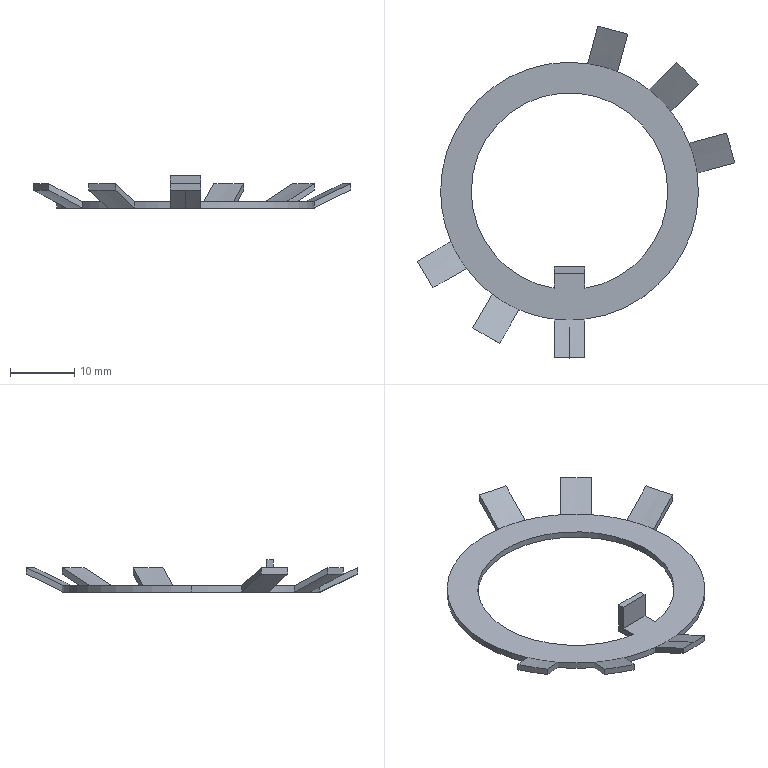Part | SolidWorks | features Boss 1, Cut 1, Revolution 1 | 1 solid | 49 faces | box 49.249 x 51.517 x 5 mm | volume 732.706 mm3 | plane 25 | cone 14 | cylinder 10 | commonest cylinder face diameters 40 x7 30.5 x3
STEP:
#1=CARTESIAN_POINT('',(0.,-20.,0.));
#2=VERTEX_POINT('',#1);
#3=CARTESIAN_POINT('',(-2.4,-19.855,0.));
#4=VERTEX_POINT('',#3);
#5=CARTESIAN_POINT('',(0.,0.,0.));
#6=DIRECTION('',(0.,0.,-1.));
#7=DIRECTION('',(0.,1.,0.));
#8=AXIS2_PLACEMENT_3D('',#5,#6,#7);
#9=CIRCLE('',#8,20.);
#10=EDGE_CURVE('',#2,#4,#9,.T.);
#11=ORIENTED_EDGE('',*,*,#10,.F.);
#12=CARTESIAN_POINT('',(0.,-25.889,2.746));
#13=VERTEX_POINT('',#12);
#14=CARTESIAN_POINT('',(0.,-20.,0.));
#15=DIRECTION('',(0.,-0.9063,0.4226));
#16=VECTOR('',#15,1000.);
#17=LINE('',#14,#16);
#18=EDGE_CURVE('',#2,#13,#17,.T.);
#19=ORIENTED_EDGE('',*,*,#18,.T.);
#20=CARTESIAN_POINT('',(-2.4,-25.889,2.798));
#21=VERTEX_POINT('',#20);
#22=CARTESIAN_POINT('',(0.,-25.889,2.746));
#23=CARTESIAN_POINT('',(-0.7991,-25.889,2.746));
#24=CARTESIAN_POINT('',(-1.6,-25.889,2.763));
#25=CARTESIAN_POINT('',(-2.4,-25.889,2.798));
#26=B_SPLINE_CURVE_WITH_KNOTS('',3,(#22,#23,#24,#25),.UNSPECIFIED.,.F.,.F.,(4,4),(0.009173,0.01157),.UNSPECIFIED.);
#27=EDGE_CURVE('',#13,#21,#26,.T.);
#28=ORIENTED_EDGE('',*,*,#27,.T.);
#29=CARTESIAN_POINT('',(-2.4,-25.889,2.798));
#30=CARTESIAN_POINT('',(-2.4,-23.878,1.864));
#31=CARTESIAN_POINT('',(-2.4,-21.867,0.9313));
#32=CARTESIAN_POINT('',(-2.4,-19.855,0.));
#33=B_SPLINE_CURVE_WITH_KNOTS('',3,(#29,#30,#31,#32),.UNSPECIFIED.,.F.,.F.,(4,4),(0.01229,0.01894),.UNSPECIFIED.);
#34=EDGE_CURVE('',#21,#4,#33,.T.);
#35=ORIENTED_EDGE('',*,*,#34,.T.);
#36=EDGE_LOOP('',(#11,#19,#28,#35));
#37=FACE_OUTER_BOUND('',#36,.T.);
#38=CARTESIAN_POINT('',(0.,0.,0.));
#39=DIRECTION('',(0.,0.,1.));
#40=DIRECTION('',(0.,-1.,0.));
#41=AXIS2_PLACEMENT_3D('',#38,#39,#40);
#42=CONICAL_SURFACE('',#41,20.,1.134);
#43=ADVANCED_FACE('',(#37),#42,.T.);
#44=CARTESIAN_POINT('',(-18.395,-7.849,1.));
#45=VERTEX_POINT('',#44);
#46=CARTESIAN_POINT('',(-20.,0.,1.));
#47=VERTEX_POINT('',#46);
#48=CARTESIAN_POINT('',(0.,0.,1.));
#49=DIRECTION('',(0.,0.,-1.));
#50=DIRECTION('',(0.,1.,0.));
#51=AXIS2_PLACEMENT_3D('',#48,#49,#50);
#52=CIRCLE('',#51,20.);
#53=EDGE_CURVE('',#45,#47,#52,.T.);
#54=ORIENTED_EDGE('',*,*,#53,.T.);
#55=CARTESIAN_POINT('',(-20.,0.,0.));
#56=VERTEX_POINT('',#55);
#57=CARTESIAN_POINT('',(-20.,0.,3.799));
#58=DIRECTION('',(0.,0.,-1.));
#59=VECTOR('',#58,1000.);
#60=LINE('',#57,#59);
#61=EDGE_CURVE('',#47,#56,#60,.T.);
#62=ORIENTED_EDGE('',*,*,#61,.T.);
#63=CARTESIAN_POINT('',(-18.395,-7.849,0.));
#64=VERTEX_POINT('',#63);
#65=CARTESIAN_POINT('',(0.,0.,0.));
#66=DIRECTION('',(0.,0.,1.));
#67=DIRECTION('',(1.,0.,0.));
#68=AXIS2_PLACEMENT_3D('',#65,#66,#67);
#69=CIRCLE('',#68,20.);
#70=EDGE_CURVE('',#56,#64,#69,.T.);
#71=ORIENTED_EDGE('',*,*,#70,.T.);
#72=CARTESIAN_POINT('',(-18.395,-7.849,3.799));
#73=DIRECTION('',(0.,0.,-1.));
#74=VECTOR('',#73,1000.);
#75=LINE('',#72,#74);
#76=EDGE_CURVE('',#45,#64,#75,.T.);
#77=ORIENTED_EDGE('',*,*,#76,.F.);
#78=EDGE_LOOP('',(#54,#62,#71,#77));
#79=FACE_OUTER_BOUND('',#78,.T.);
#80=CARTESIAN_POINT('',(0.,0.,3.799));
#81=DIRECTION('',(0.,0.,-1.));
#82=DIRECTION('',(-1.,0.,0.));
#83=AXIS2_PLACEMENT_3D('',#80,#81,#82);
#84=CYLINDRICAL_SURFACE('',#83,20.);
#85=ADVANCED_FACE('',(#79),#84,.T.);
#86=CARTESIAN_POINT('',(2.4,-15.06,1.));
#87=VERTEX_POINT('',#86);
#88=CARTESIAN_POINT('',(15.25,0.,1.));
#89=VERTEX_POINT('',#88);
#90=CARTESIAN_POINT('',(0.,0.,1.));
#91=DIRECTION('',(0.,0.,1.));
#92=DIRECTION('',(0.,-1.,0.));
#93=AXIS2_PLACEMENT_3D('',#90,#91,#92);
#94=CIRCLE('',#93,15.25);
#95=EDGE_CURVE('',#87,#89,#94,.T.);
#96=ORIENTED_EDGE('',*,*,#95,.T.);
#97=CARTESIAN_POINT('',(15.25,0.,0.));
#98=VERTEX_POINT('',#97);
#99=CARTESIAN_POINT('',(15.25,0.,3.799));
#100=DIRECTION('',(0.,0.,-1.));
#101=VECTOR('',#100,1000.);
#102=LINE('',#99,#101);
#103=EDGE_CURVE('',#89,#98,#102,.T.);
#104=ORIENTED_EDGE('',*,*,#103,.T.);
#105=CARTESIAN_POINT('',(2.4,-15.06,0.));
#106=VERTEX_POINT('',#105);
#107=CARTESIAN_POINT('',(0.,0.,0.));
#108=DIRECTION('',(0.,0.,1.));
#109=DIRECTION('',(1.,0.,0.));
#110=AXIS2_PLACEMENT_3D('',#107,#108,#109);
#111=CIRCLE('',#110,15.25);
#112=EDGE_CURVE('',#106,#98,#111,.T.);
#113=ORIENTED_EDGE('',*,*,#112,.F.);
#114=CARTESIAN_POINT('',(2.4,-15.06,3.799));
#115=DIRECTION('',(0.,0.,-1.));
#116=VECTOR('',#115,1000.);
#117=LINE('',#114,#116);
#118=EDGE_CURVE('',#87,#106,#117,.T.);
#119=ORIENTED_EDGE('',*,*,#118,.F.);
#120=EDGE_LOOP('',(#96,#104,#113,#119));
#121=FACE_OUTER_BOUND('',#120,.T.);
#122=CARTESIAN_POINT('',(0.,0.,3.799));
#123=DIRECTION('',(0.,0.,-1.));
#124=DIRECTION('',(-1.,0.,0.));
#125=AXIS2_PLACEMENT_3D('',#122,#123,#124);
#126=CYLINDRICAL_SURFACE('',#125,15.25);
#127=ADVANCED_FACE('',(#121),#126,.F.);
#128=ORIENTED_EDGE('',*,*,#103,.F.);
#129=CARTESIAN_POINT('',(-15.25,0.,1.));
#130=VERTEX_POINT('',#129);
#131=CARTESIAN_POINT('',(0.,0.,1.));
#132=DIRECTION('',(0.,0.,1.));
#133=DIRECTION('',(0.,-1.,0.));
#134=AXIS2_PLACEMENT_3D('',#131,#132,#133);
#135=CIRCLE('',#134,15.25);
#136=EDGE_CURVE('',#89,#130,#135,.T.);
#137=ORIENTED_EDGE('',*,*,#136,.T.);
#138=CARTESIAN_POINT('',(-15.25,0.,0.));
#139=VERTEX_POINT('',#138);
#140=CARTESIAN_POINT('',(-15.25,0.,3.799));
#141=DIRECTION('',(0.,0.,-1.));
#142=VECTOR('',#141,1000.);
#143=LINE('',#140,#142);
#144=EDGE_CURVE('',#130,#139,#143,.T.);
#145=ORIENTED_EDGE('',*,*,#144,.T.);
#146=CARTESIAN_POINT('',(0.,0.,0.));
#147=DIRECTION('',(0.,0.,1.));
#148=DIRECTION('',(1.,0.,0.));
#149=AXIS2_PLACEMENT_3D('',#146,#147,#148);
#150=CIRCLE('',#149,15.25);
#151=EDGE_CURVE('',#98,#139,#150,.T.);
#152=ORIENTED_EDGE('',*,*,#151,.F.);
#153=EDGE_LOOP('',(#128,#137,#145,#152));
#154=FACE_OUTER_BOUND('',#153,.T.);
#155=CARTESIAN_POINT('',(0.,0.,3.799));
#156=DIRECTION('',(0.,0.,-1.));
#157=DIRECTION('',(-1.,0.,0.));
#158=AXIS2_PLACEMENT_3D('',#155,#156,#157);
#159=CYLINDRICAL_SURFACE('',#158,15.25);
#160=ADVANCED_FACE('',(#154),#159,.F.);
#161=CARTESIAN_POINT('',(2.4,-19.855,1.));
#162=VERTEX_POINT('',#161);
#163=CARTESIAN_POINT('',(0.,-20.,1.));
#164=VERTEX_POINT('',#163);
#165=CARTESIAN_POINT('',(0.,0.,1.));
#166=DIRECTION('',(0.,0.,-1.));
#167=DIRECTION('',(0.,1.,0.));
#168=AXIS2_PLACEMENT_3D('',#165,#166,#167);
#169=CIRCLE('',#168,20.);
#170=EDGE_CURVE('',#162,#164,#169,.T.);
#171=ORIENTED_EDGE('',*,*,#170,.T.);
#172=CARTESIAN_POINT('',(0.,-25.889,3.746));
#173=VERTEX_POINT('',#172);
#174=CARTESIAN_POINT('',(0.,-26.,3.798));
#175=DIRECTION('',(0.,-0.9063,0.4226));
#176=VECTOR('',#175,1000.);
#177=LINE('',#174,#176);
#178=EDGE_CURVE('',#164,#173,#177,.T.);
#179=ORIENTED_EDGE('',*,*,#178,.T.);
#180=CARTESIAN_POINT('',(2.4,-25.889,3.798));
#181=VERTEX_POINT('',#180);
#182=CARTESIAN_POINT('',(0.,-25.889,3.746));
#183=CARTESIAN_POINT('',(0.8011,-25.889,3.746));
#184=CARTESIAN_POINT('',(1.601,-25.889,3.763));
#185=CARTESIAN_POINT('',(2.4,-25.889,3.798));
#186=B_SPLINE_CURVE_WITH_KNOTS('',3,(#182,#183,#184,#185),.UNSPECIFIED.,.F.,.F.,(4,4),(0.01271,0.01511),.UNSPECIFIED.);
#187=EDGE_CURVE('',#173,#181,#186,.T.);
#188=ORIENTED_EDGE('',*,*,#187,.T.);
#189=CARTESIAN_POINT('',(2.4,-25.889,3.798));
#190=CARTESIAN_POINT('',(2.4,-23.878,2.864));
#191=CARTESIAN_POINT('',(2.4,-21.867,1.931));
#192=CARTESIAN_POINT('',(2.4,-19.855,1.));
#193=B_SPLINE_CURVE_WITH_KNOTS('',3,(#189,#190,#191,#192),.UNSPECIFIED.,.F.,.F.,(4,4),(0.01229,0.01894),.UNSPECIFIED.);
#194=EDGE_CURVE('',#181,#162,#193,.T.);
#195=ORIENTED_EDGE('',*,*,#194,.T.);
#196=EDGE_LOOP('',(#171,#179,#188,#195));
#197=FACE_OUTER_BOUND('',#196,.T.);
#198=CARTESIAN_POINT('',(0.,0.,3.798));
#199=DIRECTION('',(0.,0.,1.));
#200=DIRECTION('',(0.,-1.,0.));
#201=AXIS2_PLACEMENT_3D('',#198,#199,#200);
#202=CONICAL_SURFACE('',#201,26.,1.134);
#203=ADVANCED_FACE('',(#197),#202,.F.);
#204=CARTESIAN_POINT('',(2.821,19.8,1.));
#205=VERTEX_POINT('',#204);
#206=CARTESIAN_POINT('',(7.457,18.558,1.));
#207=VERTEX_POINT('',#206);
#208=CARTESIAN_POINT('',(0.,0.,1.));
#209=DIRECTION('',(0.,0.,-1.));
#210=DIRECTION('',(0.,1.,0.));
#211=AXIS2_PLACEMENT_3D('',#208,#209,#210);
#212=CIRCLE('',#211,20.);
#213=EDGE_CURVE('',#205,#207,#212,.T.);
#214=ORIENTED_EDGE('',*,*,#213,.F.);
#215=CARTESIAN_POINT('',(0.,0.,1.));
#216=DIRECTION('',(0.,0.,-1.));
#217=DIRECTION('',(0.,1.,0.));
#218=AXIS2_PLACEMENT_3D('',#215,#216,#217);
#219=CIRCLE('',#218,20.);
#220=EDGE_CURVE('',#47,#205,#219,.T.);
#221=ORIENTED_EDGE('',*,*,#220,.F.);
#222=ORIENTED_EDGE('',*,*,#53,.F.);
#223=CARTESIAN_POINT('',(-15.995,-12.006,1.));
#224=VERTEX_POINT('',#223);
#225=CARTESIAN_POINT('',(0.,0.,1.));
#226=DIRECTION('',(0.,0.,-1.));
#227=DIRECTION('',(0.,1.,0.));
#228=AXIS2_PLACEMENT_3D('',#225,#226,#227);
#229=CIRCLE('',#228,20.);
#230=EDGE_CURVE('',#224,#45,#229,.T.);
#231=ORIENTED_EDGE('',*,*,#230,.F.);
#232=CARTESIAN_POINT('',(-12.006,-15.995,1.));
#233=VERTEX_POINT('',#232);
#234=CARTESIAN_POINT('',(0.,0.,1.));
#235=DIRECTION('',(0.,0.,-1.));
#236=DIRECTION('',(0.,1.,0.));
#237=AXIS2_PLACEMENT_3D('',#234,#235,#236);
#238=CIRCLE('',#237,20.);
#239=EDGE_CURVE('',#233,#224,#238,.T.);
#240=ORIENTED_EDGE('',*,*,#239,.F.);
#241=CARTESIAN_POINT('',(-7.849,-18.395,1.));
#242=VERTEX_POINT('',#241);
#243=CARTESIAN_POINT('',(0.,0.,1.));
#244=DIRECTION('',(0.,0.,-1.));
#245=DIRECTION('',(0.,1.,0.));
#246=AXIS2_PLACEMENT_3D('',#243,#244,#245);
#247=CIRCLE('',#246,20.);
#248=EDGE_CURVE('',#242,#233,#247,.T.);
#249=ORIENTED_EDGE('',*,*,#248,.F.);
#250=CARTESIAN_POINT('',(-2.4,-19.855,1.));
#251=VERTEX_POINT('',#250);
#252=CARTESIAN_POINT('',(0.,0.,1.));
#253=DIRECTION('',(0.,0.,-1.));
#254=DIRECTION('',(0.,1.,0.));
#255=AXIS2_PLACEMENT_3D('',#252,#253,#254);
#256=CIRCLE('',#255,20.);
#257=EDGE_CURVE('',#251,#242,#256,.T.);
#258=ORIENTED_EDGE('',*,*,#257,.F.);
#259=CARTESIAN_POINT('',(0.,0.,1.));
#260=DIRECTION('',(0.,0.,-1.));
#261=DIRECTION('',(0.,1.,0.));
#262=AXIS2_PLACEMENT_3D('',#259,#260,#261);
#263=CIRCLE('',#262,20.);
#264=EDGE_CURVE('',#164,#251,#263,.T.);
#265=ORIENTED_EDGE('',*,*,#264,.F.);
#266=ORIENTED_EDGE('',*,*,#170,.F.);
#267=CARTESIAN_POINT('',(19.8,2.821,1.));
#268=VERTEX_POINT('',#267);
#269=CARTESIAN_POINT('',(0.,0.,1.));
#270=DIRECTION('',(0.,0.,-1.));
#271=DIRECTION('',(0.,1.,0.));
#272=AXIS2_PLACEMENT_3D('',#269,#270,#271);
#273=CIRCLE('',#272,20.);
#274=EDGE_CURVE('',#268,#162,#273,.T.);
#275=ORIENTED_EDGE('',*,*,#274,.F.);
#276=CARTESIAN_POINT('',(18.558,7.457,1.));
#277=VERTEX_POINT('',#276);
#278=CARTESIAN_POINT('',(0.,0.,1.));
#279=DIRECTION('',(0.,0.,-1.));
#280=DIRECTION('',(0.,1.,0.));
#281=AXIS2_PLACEMENT_3D('',#278,#279,#280);
#282=CIRCLE('',#281,20.);
#283=EDGE_CURVE('',#277,#268,#282,.T.);
#284=ORIENTED_EDGE('',*,*,#283,.F.);
#285=CARTESIAN_POINT('',(15.737,12.343,1.));
#286=VERTEX_POINT('',#285);
#287=CARTESIAN_POINT('',(0.,0.,1.));
#288=DIRECTION('',(0.,0.,-1.));
#289=DIRECTION('',(0.,1.,0.));
#290=AXIS2_PLACEMENT_3D('',#287,#288,#289);
#291=CIRCLE('',#290,20.);
#292=EDGE_CURVE('',#286,#277,#291,.T.);
#293=ORIENTED_EDGE('',*,*,#292,.F.);
#294=CARTESIAN_POINT('',(12.343,15.737,1.));
#295=VERTEX_POINT('',#294);
#296=CARTESIAN_POINT('',(0.,0.,1.));
#297=DIRECTION('',(0.,0.,-1.));
#298=DIRECTION('',(0.,1.,0.));
#299=AXIS2_PLACEMENT_3D('',#296,#297,#298);
#300=CIRCLE('',#299,20.);
#301=EDGE_CURVE('',#295,#286,#300,.T.);
#302=ORIENTED_EDGE('',*,*,#301,.F.);
#303=CARTESIAN_POINT('',(0.,0.,1.));
#304=DIRECTION('',(0.,0.,-1.));
#305=DIRECTION('',(0.,1.,0.));
#306=AXIS2_PLACEMENT_3D('',#303,#304,#305);
#307=CIRCLE('',#306,20.);
#308=EDGE_CURVE('',#207,#295,#307,.T.);
#309=ORIENTED_EDGE('',*,*,#308,.F.);
#310=EDGE_LOOP('',(#214,#221,#222,#231,#240,#249,#258,#265,#266,#275,#284,#293,#302,#309));
#311=FACE_OUTER_BOUND('',#310,.T.);
#312=CARTESIAN_POINT('',(2.4,-12.75,1.));
#313=VERTEX_POINT('',#312);
#314=CARTESIAN_POINT('',(2.4,-15.06,1.));
#315=DIRECTION('',(0.,-1.,0.));
#316=VECTOR('',#315,1000.);
#317=LINE('',#314,#316);
#318=EDGE_CURVE('',#313,#87,#317,.T.);
#319=ORIENTED_EDGE('',*,*,#318,.F.);
#320=CARTESIAN_POINT('',(-2.4,-12.75,1.));
#321=VERTEX_POINT('',#320);
#322=CARTESIAN_POINT('',(0.,-12.75,1.));
#323=DIRECTION('',(-1.,0.,0.));
#324=VECTOR('',#323,1000.);
#325=LINE('',#322,#324);
#326=EDGE_CURVE('',#313,#321,#325,.T.);
#327=ORIENTED_EDGE('',*,*,#326,.T.);
#328=CARTESIAN_POINT('',(-2.4,-15.06,1.));
#329=VERTEX_POINT('',#328);
#330=CARTESIAN_POINT('',(-2.4,-15.06,1.));
#331=DIRECTION('',(0.,1.,0.));
#332=VECTOR('',#331,1000.);
#333=LINE('',#330,#332);
#334=EDGE_CURVE('',#329,#321,#333,.T.);
#335=ORIENTED_EDGE('',*,*,#334,.F.);
#336=CARTESIAN_POINT('',(0.,0.,1.));
#337=DIRECTION('',(0.,0.,1.));
#338=DIRECTION('',(0.,-1.,0.));
#339=AXIS2_PLACEMENT_3D('',#336,#337,#338);
#340=CIRCLE('',#339,15.25);
#341=EDGE_CURVE('',#130,#329,#340,.T.);
#342=ORIENTED_EDGE('',*,*,#341,.F.);
#343=ORIENTED_EDGE('',*,*,#136,.F.);
#344=ORIENTED_EDGE('',*,*,#95,.F.);
#345=EDGE_LOOP('',(#319,#327,#335,#342,#343,#344));
#346=FACE_BOUND('',#345,.T.);
#347=CARTESIAN_POINT('',(0.,20.,1.));
#348=DIRECTION('',(0.,0.,1.));
#349=DIRECTION('',(0.,-1.,0.));
#350=AXIS2_PLACEMENT_3D('',#347,#348,#349);
#351=PLANE('',#350);
#352=ADVANCED_FACE('',(#311,#346),#351,.T.);
#353=ORIENTED_EDGE('',*,*,#178,.F.);
#354=ORIENTED_EDGE('',*,*,#264,.T.);
#355=CARTESIAN_POINT('',(-2.4,-25.889,3.798));
#356=VERTEX_POINT('',#355);
#357=CARTESIAN_POINT('',(-2.4,-19.855,1.));
#358=CARTESIAN_POINT('',(-2.4,-21.867,1.931));
#359=CARTESIAN_POINT('',(-2.4,-23.878,2.864));
#360=CARTESIAN_POINT('',(-2.4,-25.889,3.798));
#361=B_SPLINE_CURVE_WITH_KNOTS('',3,(#357,#358,#359,#360),.UNSPECIFIED.,.F.,.F.,(4,4),(0.007598,0.01425),.UNSPECIFIED.);
#362=EDGE_CURVE('',#251,#356,#361,.T.);
#363=ORIENTED_EDGE('',*,*,#362,.T.);
#364=CARTESIAN_POINT('',(-2.4,-25.889,3.798));
#365=CARTESIAN_POINT('',(-1.6,-25.889,3.763));
#366=CARTESIAN_POINT('',(-0.7991,-25.889,3.746));
#367=CARTESIAN_POINT('',(0.,-25.889,3.746));
#368=B_SPLINE_CURVE_WITH_KNOTS('',3,(#364,#365,#366,#367),.UNSPECIFIED.,.F.,.F.,(4,4),(0.01032,0.01271),.UNSPECIFIED.);
#369=EDGE_CURVE('',#356,#173,#368,.T.);
#370=ORIENTED_EDGE('',*,*,#369,.T.);
#371=EDGE_LOOP('',(#353,#354,#363,#370));
#372=FACE_OUTER_BOUND('',#371,.T.);
#373=CARTESIAN_POINT('',(0.,0.,3.798));
#374=DIRECTION('',(0.,0.,1.));
#375=DIRECTION('',(0.,-1.,0.));
#376=AXIS2_PLACEMENT_3D('',#373,#374,#375);
#377=CONICAL_SURFACE('',#376,26.,1.134);
#378=ADVANCED_FACE('',(#372),#377,.F.);
#379=CARTESIAN_POINT('',(-15.023,-21.221,3.798));
#380=VERTEX_POINT('',#379);
#381=CARTESIAN_POINT('',(-12.006,-15.995,1.));
#382=CARTESIAN_POINT('',(-13.012,-17.738,1.931));
#383=CARTESIAN_POINT('',(-14.018,-19.479,2.864));
#384=CARTESIAN_POINT('',(-15.023,-21.221,3.798));
#385=B_SPLINE_CURVE_WITH_KNOTS('',3,(#381,#382,#383,#384),.UNSPECIFIED.,.F.,.F.,(4,4),(0.000000255,0.006651),.UNSPECIFIED.);
#386=EDGE_CURVE('',#233,#380,#385,.T.);
#387=ORIENTED_EDGE('',*,*,#386,.T.);
#388=CARTESIAN_POINT('',(-10.866,-23.621,3.798));
#389=VERTEX_POINT('',#388);
#390=CARTESIAN_POINT('',(-15.023,-21.221,3.798));
#391=CARTESIAN_POINT('',(-13.637,-22.021,3.729));
#392=CARTESIAN_POINT('',(-12.252,-22.821,3.729));
#393=CARTESIAN_POINT('',(-10.866,-23.621,3.798));
#394=B_SPLINE_CURVE_WITH_KNOTS('',3,(#390,#391,#392,#393),.UNSPECIFIED.,.F.,.F.,(4,4),(0.000000231,0.0048),.UNSPECIFIED.);
#395=EDGE_CURVE('',#380,#389,#394,.T.);
#396=ORIENTED_EDGE('',*,*,#395,.T.);
#397=CARTESIAN_POINT('',(-10.866,-23.621,3.798));
#398=CARTESIAN_POINT('',(-9.861,-21.879,2.864));
#399=CARTESIAN_POINT('',(-8.855,-20.138,1.931));
#400=CARTESIAN_POINT('',(-7.849,-18.395,1.));
#401=B_SPLINE_CURVE_WITH_KNOTS('',3,(#397,#398,#399,#400),.UNSPECIFIED.,.F.,.F.,(4,4),(0.000000255,0.006651),.UNSPECIFIED.);
#402=EDGE_CURVE('',#389,#242,#401,.T.);
#403=ORIENTED_EDGE('',*,*,#402,.T.);
#404=ORIENTED_EDGE('',*,*,#248,.T.);
#405=EDGE_LOOP('',(#387,#396,#403,#404));
#406=FACE_OUTER_BOUND('',#405,.T.);
#407=CARTESIAN_POINT('',(0.,0.,3.798));
#408=DIRECTION('',(0.,0.,1.));
#409=DIRECTION('',(0.,-1.,0.));
#410=AXIS2_PLACEMENT_3D('',#407,#408,#409);
#411=CONICAL_SURFACE('',#410,26.,1.134);
#412=ADVANCED_FACE('',(#406),#411,.F.);
#413=CARTESIAN_POINT('',(-23.621,-10.866,3.798));
#414=VERTEX_POINT('',#413);
#415=CARTESIAN_POINT('',(-18.395,-7.849,1.));
#416=CARTESIAN_POINT('',(-20.138,-8.855,1.931));
#417=CARTESIAN_POINT('',(-21.879,-9.861,2.864));
#418=CARTESIAN_POINT('',(-23.621,-10.866,3.798));
#419=B_SPLINE_CURVE_WITH_KNOTS('',3,(#415,#416,#417,#418),.UNSPECIFIED.,.F.,.F.,(4,4),(0.000000255,0.006651),.UNSPECIFIED.);
#420=EDGE_CURVE('',#45,#414,#419,.T.);
#421=ORIENTED_EDGE('',*,*,#420,.T.);
#422=CARTESIAN_POINT('',(-21.221,-15.023,3.798));
#423=VERTEX_POINT('',#422);
#424=CARTESIAN_POINT('',(-23.621,-10.866,3.798));
#425=CARTESIAN_POINT('',(-22.821,-12.252,3.729));
#426=CARTESIAN_POINT('',(-22.021,-13.637,3.729));
#427=CARTESIAN_POINT('',(-21.221,-15.023,3.798));
#428=B_SPLINE_CURVE_WITH_KNOTS('',3,(#424,#425,#426,#427),.UNSPECIFIED.,.F.,.F.,(4,4),(0.000000231,0.0048),.UNSPECIFIED.);
#429=EDGE_CURVE('',#414,#423,#428,.T.);
#430=ORIENTED_EDGE('',*,*,#429,.T.);
#431=CARTESIAN_POINT('',(-21.221,-15.023,3.798));
#432=CARTESIAN_POINT('',(-19.479,-14.018,2.864));
#433=CARTESIAN_POINT('',(-17.738,-13.012,1.931));
#434=CARTESIAN_POINT('',(-15.995,-12.006,1.));
#435=B_SPLINE_CURVE_WITH_KNOTS('',3,(#431,#432,#433,#434),.UNSPECIFIED.,.F.,.F.,(4,4),(0.000000255,0.006651),.UNSPECIFIED.);
#436=EDGE_CURVE('',#423,#224,#435,.T.);
#437=ORIENTED_EDGE('',*,*,#436,.T.);
#438=ORIENTED_EDGE('',*,*,#230,.T.);
#439=EDGE_LOOP('',(#421,#430,#437,#438));
#440=FACE_OUTER_BOUND('',#439,.T.);
#441=CARTESIAN_POINT('',(0.,0.,3.798));
#442=DIRECTION('',(0.,0.,1.));
#443=DIRECTION('',(0.,-1.,0.));
#444=AXIS2_PLACEMENT_3D('',#441,#442,#443);
#445=CONICAL_SURFACE('',#444,26.,1.134);
#446=ADVANCED_FACE('',(#440),#445,.F.);
#447=CARTESIAN_POINT('',(9.019,24.386,3.798));
#448=VERTEX_POINT('',#447);
#449=CARTESIAN_POINT('',(7.457,18.558,1.));
#450=CARTESIAN_POINT('',(7.978,20.501,1.931));
#451=CARTESIAN_POINT('',(8.498,22.443,2.864));
#452=CARTESIAN_POINT('',(9.019,24.386,3.798));
#453=B_SPLINE_CURVE_WITH_KNOTS('',3,(#449,#450,#451,#452),.UNSPECIFIED.,.F.,.F.,(4,4),(0.000000228,0.006651),.UNSPECIFIED.);
#454=EDGE_CURVE('',#207,#448,#453,.T.);
#455=ORIENTED_EDGE('',*,*,#454,.T.);
#456=CARTESIAN_POINT('',(4.382,25.628,3.798));
#457=VERTEX_POINT('',#456);
#458=CARTESIAN_POINT('',(9.019,24.386,3.798));
#459=CARTESIAN_POINT('',(7.473,24.8,3.729));
#460=CARTESIAN_POINT('',(5.928,25.214,3.729));
#461=CARTESIAN_POINT('',(4.382,25.628,3.798));
#462=B_SPLINE_CURVE_WITH_KNOTS('',3,(#458,#459,#460,#461),.UNSPECIFIED.,.F.,.F.,(4,4),(0.000000207,0.0048),.UNSPECIFIED.);
#463=EDGE_CURVE('',#448,#457,#462,.T.);
#464=ORIENTED_EDGE('',*,*,#463,.T.);
#465=CARTESIAN_POINT('',(4.382,25.628,3.798));
#466=CARTESIAN_POINT('',(3.862,23.686,2.864));
#467=CARTESIAN_POINT('',(3.341,21.743,1.931));
#468=CARTESIAN_POINT('',(2.821,19.8,1.));
#469=B_SPLINE_CURVE_WITH_KNOTS('',3,(#465,#466,#467,#468),.UNSPECIFIED.,.F.,.F.,(4,4),(0.000000228,0.006651),.UNSPECIFIED.);
#470=EDGE_CURVE('',#457,#205,#469,.T.);
#471=ORIENTED_EDGE('',*,*,#470,.T.);
#472=ORIENTED_EDGE('',*,*,#213,.T.);
#473=EDGE_LOOP('',(#455,#464,#471,#472));
#474=FACE_OUTER_BOUND('',#473,.T.);
#475=CARTESIAN_POINT('',(0.,0.,3.798));
#476=DIRECTION('',(0.,0.,1.));
#477=DIRECTION('',(0.,-1.,0.));
#478=AXIS2_PLACEMENT_3D('',#475,#476,#477);
#479=CONICAL_SURFACE('',#478,26.,1.134);
#480=ADVANCED_FACE('',(#474),#479,.F.);
#481=CARTESIAN_POINT('',(20.003,16.609,3.798));
#482=VERTEX_POINT('',#481);
#483=CARTESIAN_POINT('',(15.737,12.343,1.));
#484=CARTESIAN_POINT('',(17.16,13.765,1.931));
#485=CARTESIAN_POINT('',(18.582,15.187,2.864));
#486=CARTESIAN_POINT('',(20.003,16.609,3.798));
#487=B_SPLINE_CURVE_WITH_KNOTS('',3,(#483,#484,#485,#486),.UNSPECIFIED.,.F.,.F.,(4,4),(0.000000312,0.006651),.UNSPECIFIED.);
#488=EDGE_CURVE('',#286,#482,#487,.T.);
#489=ORIENTED_EDGE('',*,*,#488,.T.);
#490=CARTESIAN_POINT('',(16.609,20.003,3.798));
#491=VERTEX_POINT('',#490);
#492=CARTESIAN_POINT('',(20.003,16.609,3.798));
#493=CARTESIAN_POINT('',(18.872,17.741,3.729));
#494=CARTESIAN_POINT('',(17.741,18.872,3.729));
#495=CARTESIAN_POINT('',(16.609,20.003,3.798));
#496=B_SPLINE_CURVE_WITH_KNOTS('',3,(#492,#493,#494,#495),.UNSPECIFIED.,.F.,.F.,(4,4),(0.000000283,0.0048),.UNSPECIFIED.);
#497=EDGE_CURVE('',#482,#491,#496,.T.);
#498=ORIENTED_EDGE('',*,*,#497,.T.);
#499=CARTESIAN_POINT('',(16.609,20.003,3.798));
#500=CARTESIAN_POINT('',(15.187,18.582,2.864));
#501=CARTESIAN_POINT('',(13.765,17.16,1.931));
#502=CARTESIAN_POINT('',(12.343,15.737,1.));
#503=B_SPLINE_CURVE_WITH_KNOTS('',3,(#499,#500,#501,#502),.UNSPECIFIED.,.F.,.F.,(4,4),(0.000000312,0.006651),.UNSPECIFIED.);
#504=EDGE_CURVE('',#491,#295,#503,.T.);
#505=ORIENTED_EDGE('',*,*,#504,.T.);
#506=ORIENTED_EDGE('',*,*,#301,.T.);
#507=EDGE_LOOP('',(#489,#498,#505,#506));
#508=FACE_OUTER_BOUND('',#507,.T.);
#509=CARTESIAN_POINT('',(0.,0.,3.798));
#510=DIRECTION('',(0.,0.,1.));
#511=DIRECTION('',(0.,-1.,0.));
#512=AXIS2_PLACEMENT_3D('',#509,#510,#511);
#513=CONICAL_SURFACE('',#512,26.,1.134);
#514=ADVANCED_FACE('',(#508),#513,.F.);
#515=CARTESIAN_POINT('',(25.628,4.382,3.798));
#516=VERTEX_POINT('',#515);
#517=CARTESIAN_POINT('',(19.8,2.821,1.));
#518=CARTESIAN_POINT('',(21.743,3.341,1.931));
#519=CARTESIAN_POINT('',(23.686,3.862,2.864));
#520=CARTESIAN_POINT('',(25.628,4.382,3.798));
#521=B_SPLINE_CURVE_WITH_KNOTS('',3,(#517,#518,#519,#520),.UNSPECIFIED.,.F.,.F.,(4,4),(0.000000228,0.006651),.UNSPECIFIED.);
#522=EDGE_CURVE('',#268,#516,#521,.T.);
#523=ORIENTED_EDGE('',*,*,#522,.T.);
#524=CARTESIAN_POINT('',(24.386,9.019,3.798));
#525=VERTEX_POINT('',#524);
#526=CARTESIAN_POINT('',(25.628,4.382,3.798));
#527=CARTESIAN_POINT('',(25.214,5.928,3.729));
#528=CARTESIAN_POINT('',(24.8,7.473,3.729));
#529=CARTESIAN_POINT('',(24.386,9.019,3.798));
#530=B_SPLINE_CURVE_WITH_KNOTS('',3,(#526,#527,#528,#529),.UNSPECIFIED.,.F.,.F.,(4,4),(0.000000207,0.0048),.UNSPECIFIED.);
#531=EDGE_CURVE('',#516,#525,#530,.T.);
#532=ORIENTED_EDGE('',*,*,#531,.T.);
#533=CARTESIAN_POINT('',(24.386,9.019,3.798));
#534=CARTESIAN_POINT('',(22.443,8.498,2.864));
#535=CARTESIAN_POINT('',(20.501,7.978,1.931));
#536=CARTESIAN_POINT('',(18.558,7.457,1.));
#537=B_SPLINE_CURVE_WITH_KNOTS('',3,(#533,#534,#535,#536),.UNSPECIFIED.,.F.,.F.,(4,4),(0.000000228,0.006651),.UNSPECIFIED.);
#538=EDGE_CURVE('',#525,#277,#537,.T.);
#539=ORIENTED_EDGE('',*,*,#538,.T.);
#540=ORIENTED_EDGE('',*,*,#283,.T.);
#541=EDGE_LOOP('',(#523,#532,#539,#540));
#542=FACE_OUTER_BOUND('',#541,.T.);
#543=CARTESIAN_POINT('',(0.,0.,3.798));
#544=DIRECTION('',(0.,0.,1.));
#545=DIRECTION('',(0.,-1.,0.));
#546=AXIS2_PLACEMENT_3D('',#543,#544,#545);
#547=CONICAL_SURFACE('',#546,26.,1.134);
#548=ADVANCED_FACE('',(#542),#547,.F.);
#549=CARTESIAN_POINT('',(2.4,-11.75,5.));
#550=VERTEX_POINT('',#549);
#551=CARTESIAN_POINT('',(2.4,-11.75,0.));
#552=VERTEX_POINT('',#551);
#553=CARTESIAN_POINT('',(2.4,-11.75,3.799));
#554=DIRECTION('',(0.,0.,-1.));
#555=VECTOR('',#554,1000.);
#556=LINE('',#553,#555);
#557=EDGE_CURVE('',#550,#552,#556,.T.);
#558=ORIENTED_EDGE('',*,*,#557,.F.);
#559=CARTESIAN_POINT('',(2.4,-12.75,5.));
#560=VERTEX_POINT('',#559);
#561=CARTESIAN_POINT('',(2.4,-11.75,5.));
#562=DIRECTION('',(0.,1.,0.));
#563=VECTOR('',#562,1000.);
#564=LINE('',#561,#563);
#565=EDGE_CURVE('',#560,#550,#564,.T.);
#566=ORIENTED_EDGE('',*,*,#565,.F.);
#567=CARTESIAN_POINT('',(2.4,-12.75,5.));
#568=DIRECTION('',(0.,0.,-1.));
#569=VECTOR('',#568,1000.);
#570=LINE('',#567,#569);
#571=EDGE_CURVE('',#560,#313,#570,.T.);
#572=ORIENTED_EDGE('',*,*,#571,.T.);
#573=ORIENTED_EDGE('',*,*,#318,.T.);
#574=ORIENTED_EDGE('',*,*,#118,.T.);
#575=CARTESIAN_POINT('',(2.4,-15.06,0.));
#576=DIRECTION('',(0.,-1.,0.));
#577=VECTOR('',#576,1000.);
#578=LINE('',#575,#577);
#579=EDGE_CURVE('',#552,#106,#578,.T.);
#580=ORIENTED_EDGE('',*,*,#579,.F.);
#581=EDGE_LOOP('',(#558,#566,#572,#573,#574,#580));
#582=FACE_OUTER_BOUND('',#581,.T.);
#583=CARTESIAN_POINT('',(2.4,-15.06,3.799));
#584=DIRECTION('',(1.,0.,0.));
#585=DIRECTION('',(0.,0.,-1.));
#586=AXIS2_PLACEMENT_3D('',#583,#584,#585);
#587=PLANE('',#586);
#588=ADVANCED_FACE('',(#582),#587,.T.);
#589=CARTESIAN_POINT('',(-2.4,-11.75,5.));
#590=VERTEX_POINT('',#589);
#591=CARTESIAN_POINT('',(-2.4,-11.75,0.));
#592=VERTEX_POINT('',#591);
#593=CARTESIAN_POINT('',(-2.4,-11.75,3.799));
#594=DIRECTION('',(0.,0.,-1.));
#595=VECTOR('',#594,1000.);
#596=LINE('',#593,#595);
#597=EDGE_CURVE('',#590,#592,#596,.T.);
#598=ORIENTED_EDGE('',*,*,#597,.F.);
#599=CARTESIAN_POINT('',(-2.4,-11.75,5.));
#600=DIRECTION('',(-1.,0.,0.));
#601=VECTOR('',#600,1000.);
#602=LINE('',#599,#601);
#603=EDGE_CURVE('',#550,#590,#602,.T.);
#604=ORIENTED_EDGE('',*,*,#603,.F.);
#605=ORIENTED_EDGE('',*,*,#557,.T.);
#606=CARTESIAN_POINT('',(2.4,-11.75,0.));
#607=DIRECTION('',(1.,0.,0.));
#608=VECTOR('',#607,1000.);
#609=LINE('',#606,#608);
#610=EDGE_CURVE('',#592,#552,#609,.T.);
#611=ORIENTED_EDGE('',*,*,#610,.F.);
#612=EDGE_LOOP('',(#598,#604,#605,#611));
#613=FACE_OUTER_BOUND('',#612,.T.);
#614=CARTESIAN_POINT('',(2.4,-11.75,3.799));
#615=DIRECTION('',(0.,1.,0.));
#616=DIRECTION('',(0.,0.,1.));
#617=AXIS2_PLACEMENT_3D('',#614,#615,#616);
#618=PLANE('',#617);
#619=ADVANCED_FACE('',(#613),#618,.T.);
#620=ORIENTED_EDGE('',*,*,#597,.T.);
#621=CARTESIAN_POINT('',(-2.4,-15.06,0.));
#622=VERTEX_POINT('',#621);
#623=CARTESIAN_POINT('',(-2.4,-15.06,0.));
#624=DIRECTION('',(0.,1.,0.));
#625=VECTOR('',#624,1000.);
#626=LINE('',#623,#625);
#627=EDGE_CURVE('',#622,#592,#626,.T.);
#628=ORIENTED_EDGE('',*,*,#627,.F.);
#629=CARTESIAN_POINT('',(-2.4,-15.06,3.799));
#630=DIRECTION('',(0.,0.,-1.));
#631=VECTOR('',#630,1000.);
#632=LINE('',#629,#631);
#633=EDGE_CURVE('',#329,#622,#632,.T.);
#634=ORIENTED_EDGE('',*,*,#633,.F.);
#635=ORIENTED_EDGE('',*,*,#334,.T.);
#636=CARTESIAN_POINT('',(-2.4,-12.75,5.));
#637=VERTEX_POINT('',#636);
#638=CARTESIAN_POINT('',(-2.4,-12.75,5.));
#639=DIRECTION('',(0.,0.,-1.));
#640=VECTOR('',#639,1000.);
#641=LINE('',#638,#640);
#642=EDGE_CURVE('',#637,#321,#641,.T.);
#643=ORIENTED_EDGE('',*,*,#642,.F.);
#644=CARTESIAN_POINT('',(-2.4,-11.75,5.));
#645=DIRECTION('',(0.,-1.,0.));
#646=VECTOR('',#645,1000.);
#647=LINE('',#644,#646);
#648=EDGE_CURVE('',#590,#637,#647,.T.);
#649=ORIENTED_EDGE('',*,*,#648,.F.);
#650=EDGE_LOOP('',(#620,#628,#634,#635,#643,#649));
#651=FACE_OUTER_BOUND('',#650,.T.);
#652=CARTESIAN_POINT('',(-2.4,-15.06,3.799));
#653=DIRECTION('',(-1.,0.,0.));
#654=DIRECTION('',(0.,-1.,0.));
#655=AXIS2_PLACEMENT_3D('',#652,#653,#654);
#656=PLANE('',#655);
#657=ADVANCED_FACE('',(#651),#656,.T.);
#658=ORIENTED_EDGE('',*,*,#144,.F.);
#659=ORIENTED_EDGE('',*,*,#341,.T.);
#660=ORIENTED_EDGE('',*,*,#633,.T.);
#661=CARTESIAN_POINT('',(0.,0.,0.));
#662=DIRECTION('',(0.,0.,1.));
#663=DIRECTION('',(1.,0.,0.));
#664=AXIS2_PLACEMENT_3D('',#661,#662,#663);
#665=CIRCLE('',#664,15.25);
#666=EDGE_CURVE('',#139,#622,#665,.T.);
#667=ORIENTED_EDGE('',*,*,#666,.F.);
#668=EDGE_LOOP('',(#658,#659,#660,#667));
#669=FACE_OUTER_BOUND('',#668,.T.);
#670=CARTESIAN_POINT('',(0.,0.,3.799));
#671=DIRECTION('',(0.,0.,-1.));
#672=DIRECTION('',(-1.,0.,0.));
#673=AXIS2_PLACEMENT_3D('',#670,#671,#672);
#674=CYLINDRICAL_SURFACE('',#673,15.25);
#675=ADVANCED_FACE('',(#669),#674,.F.);
#676=CARTESIAN_POINT('',(2.4,-19.855,0.));
#677=VERTEX_POINT('',#676);
#678=CARTESIAN_POINT('',(2.4,-25.889,2.798));
#679=VERTEX_POINT('',#678);
#680=CARTESIAN_POINT('',(2.4,-19.855,0.));
#681=CARTESIAN_POINT('',(2.4,-21.867,0.9313));
#682=CARTESIAN_POINT('',(2.4,-23.878,1.864));
#683=CARTESIAN_POINT('',(2.4,-25.889,2.798));
#684=B_SPLINE_CURVE_WITH_KNOTS('',3,(#680,#681,#682,#683),.UNSPECIFIED.,.F.,.F.,(4,4),(0.007598,0.01425),.UNSPECIFIED.);
#685=EDGE_CURVE('',#677,#679,#684,.T.);
#686=ORIENTED_EDGE('',*,*,#685,.F.);
#687=CARTESIAN_POINT('',(2.4,-19.855,3.799));
#688=DIRECTION('',(0.,0.,-1.));
#689=VECTOR('',#688,1000.);
#690=LINE('',#687,#689);
#691=EDGE_CURVE('',#162,#677,#690,.T.);
#692=ORIENTED_EDGE('',*,*,#691,.F.);
#693=ORIENTED_EDGE('',*,*,#194,.F.);
#694=CARTESIAN_POINT('',(2.4,-25.889,3.799));
#695=DIRECTION('',(0.,0.,-1.));
#696=VECTOR('',#695,1000.);
#697=LINE('',#694,#696);
#698=EDGE_CURVE('',#181,#679,#697,.T.);
#699=ORIENTED_EDGE('',*,*,#698,.T.);
#700=EDGE_LOOP('',(#686,#692,#693,#699));
#701=FACE_OUTER_BOUND('',#700,.T.);
#702=CARTESIAN_POINT('',(2.4,-19.855,3.799));
#703=DIRECTION('',(-1.,0.,0.));
#704=DIRECTION('',(0.,-1.,0.));
#705=AXIS2_PLACEMENT_3D('',#702,#703,#704);
#706=PLANE('',#705);
#707=ADVANCED_FACE('',(#701),#706,.F.);
#708=ORIENTED_EDGE('',*,*,#274,.T.);
#709=ORIENTED_EDGE('',*,*,#691,.T.);
#710=CARTESIAN_POINT('',(19.8,2.821,0.));
#711=VERTEX_POINT('',#710);
#712=CARTESIAN_POINT('',(0.,0.,0.));
#713=DIRECTION('',(0.,0.,1.));
#714=DIRECTION('',(1.,0.,0.));
#715=AXIS2_PLACEMENT_3D('',#712,#713,#714);
#716=CIRCLE('',#715,20.);
#717=EDGE_CURVE('',#677,#711,#716,.T.);
#718=ORIENTED_EDGE('',*,*,#717,.T.);
#719=CARTESIAN_POINT('',(19.8,2.821,3.799));
#720=DIRECTION('',(0.,0.,-1.));
#721=VECTOR('',#720,1000.);
#722=LINE('',#719,#721);
#723=EDGE_CURVE('',#268,#711,#722,.T.);
#724=ORIENTED_EDGE('',*,*,#723,.F.);
#725=EDGE_LOOP('',(#708,#709,#718,#724));
#726=FACE_OUTER_BOUND('',#725,.T.);
#727=CARTESIAN_POINT('',(0.,0.,3.799));
#728=DIRECTION('',(0.,0.,-1.));
#729=DIRECTION('',(-1.,0.,0.));
#730=AXIS2_PLACEMENT_3D('',#727,#728,#729);
#731=CYLINDRICAL_SURFACE('',#730,20.);
#732=ADVANCED_FACE('',(#726),#731,.T.);
#733=CARTESIAN_POINT('',(25.628,4.382,2.798));
#734=VERTEX_POINT('',#733);
#735=CARTESIAN_POINT('',(25.628,4.382,2.798));
#736=CARTESIAN_POINT('',(23.686,3.862,1.864));
#737=CARTESIAN_POINT('',(21.743,3.341,0.9313));
#738=CARTESIAN_POINT('',(19.8,2.821,0.));
#739=B_SPLINE_CURVE_WITH_KNOTS('',3,(#735,#736,#737,#738),.UNSPECIFIED.,.F.,.F.,(4,4),(0.000000228,0.006651),.UNSPECIFIED.);
#740=EDGE_CURVE('',#734,#711,#739,.T.);
#741=ORIENTED_EDGE('',*,*,#740,.F.);
#742=CARTESIAN_POINT('',(25.628,4.382,3.799));
#743=DIRECTION('',(0.,0.,-1.));
#744=VECTOR('',#743,1000.);
#745=LINE('',#742,#744);
#746=EDGE_CURVE('',#516,#734,#745,.T.);
#747=ORIENTED_EDGE('',*,*,#746,.F.);
#748=ORIENTED_EDGE('',*,*,#522,.F.);
#749=ORIENTED_EDGE('',*,*,#723,.T.);
#750=EDGE_LOOP('',(#741,#747,#748,#749));
#751=FACE_OUTER_BOUND('',#750,.T.);
#752=CARTESIAN_POINT('',(19.8,2.821,3.799));
#753=DIRECTION('',(-0.2588,0.9659,0.));
#754=DIRECTION('',(-0.9659,-0.2588,0.));
#755=AXIS2_PLACEMENT_3D('',#752,#753,#754);
#756=PLANE('',#755);
#757=ADVANCED_FACE('',(#751),#756,.F.);
#758=CARTESIAN_POINT('',(24.386,9.019,2.798));
#759=VERTEX_POINT('',#758);
#760=CARTESIAN_POINT('',(24.386,9.019,2.798));
#761=CARTESIAN_POINT('',(24.8,7.473,2.729));
#762=CARTESIAN_POINT('',(25.214,5.928,2.729));
#763=CARTESIAN_POINT('',(25.628,4.382,2.798));
#764=B_SPLINE_CURVE_WITH_KNOTS('',3,(#760,#761,#762,#763),.UNSPECIFIED.,.F.,.F.,(4,4),(0.000000207,0.0048),.UNSPECIFIED.);
#765=EDGE_CURVE('',#759,#734,#764,.T.);
#766=ORIENTED_EDGE('',*,*,#765,.F.);
#767=CARTESIAN_POINT('',(24.386,9.019,3.799));
#768=DIRECTION('',(0.,0.,-1.));
#769=VECTOR('',#768,1000.);
#770=LINE('',#767,#769);
#771=EDGE_CURVE('',#525,#759,#770,.T.);
#772=ORIENTED_EDGE('',*,*,#771,.F.);
#773=ORIENTED_EDGE('',*,*,#531,.F.);
#774=ORIENTED_EDGE('',*,*,#746,.T.);
#775=EDGE_LOOP('',(#766,#772,#773,#774));
#776=FACE_OUTER_BOUND('',#775,.T.);
#777=CARTESIAN_POINT('',(24.386,9.019,3.799));
#778=DIRECTION('',(-0.9659,-0.2588,0.));
#779=DIRECTION('',(0.2588,-0.9659,0.));
#780=AXIS2_PLACEMENT_3D('',#777,#778,#779);
#781=PLANE('',#780);
#782=ADVANCED_FACE('',(#776),#781,.F.);
#783=CARTESIAN_POINT('',(18.558,7.457,0.));
#784=VERTEX_POINT('',#783);
#785=CARTESIAN_POINT('',(18.558,7.457,0.));
#786=CARTESIAN_POINT('',(20.501,7.978,0.9313));
#787=CARTESIAN_POINT('',(22.443,8.498,1.864));
#788=CARTESIAN_POINT('',(24.386,9.019,2.798));
#789=B_SPLINE_CURVE_WITH_KNOTS('',3,(#785,#786,#787,#788),.UNSPECIFIED.,.F.,.F.,(4,4),(0.000000228,0.006651),.UNSPECIFIED.);
#790=EDGE_CURVE('',#784,#759,#789,.T.);
#791=ORIENTED_EDGE('',*,*,#790,.F.);
#792=CARTESIAN_POINT('',(18.558,7.457,3.799));
#793=DIRECTION('',(0.,0.,-1.));
#794=VECTOR('',#793,1000.);
#795=LINE('',#792,#794);
#796=EDGE_CURVE('',#277,#784,#795,.T.);
#797=ORIENTED_EDGE('',*,*,#796,.F.);
#798=ORIENTED_EDGE('',*,*,#538,.F.);
#799=ORIENTED_EDGE('',*,*,#771,.T.);
#800=EDGE_LOOP('',(#791,#797,#798,#799));
#801=FACE_OUTER_BOUND('',#800,.T.);
#802=CARTESIAN_POINT('',(18.558,7.457,3.799));
#803=DIRECTION('',(0.2588,-0.9659,0.));
#804=DIRECTION('',(0.9659,0.2588,0.));
#805=AXIS2_PLACEMENT_3D('',#802,#803,#804);
#806=PLANE('',#805);
#807=ADVANCED_FACE('',(#801),#806,.F.);
#808=ORIENTED_EDGE('',*,*,#292,.T.);
#809=ORIENTED_EDGE('',*,*,#796,.T.);
#810=CARTESIAN_POINT('',(15.737,12.343,0.));
#811=VERTEX_POINT('',#810);
#812=CARTESIAN_POINT('',(0.,0.,0.));
#813=DIRECTION('',(0.,0.,1.));
#814=DIRECTION('',(1.,0.,0.));
#815=AXIS2_PLACEMENT_3D('',#812,#813,#814);
#816=CIRCLE('',#815,20.);
#817=EDGE_CURVE('',#784,#811,#816,.T.);
#818=ORIENTED_EDGE('',*,*,#817,.T.);
#819=CARTESIAN_POINT('',(15.737,12.343,3.799));
#820=DIRECTION('',(0.,0.,-1.));
#821=VECTOR('',#820,1000.);
#822=LINE('',#819,#821);
#823=EDGE_CURVE('',#286,#811,#822,.T.);
#824=ORIENTED_EDGE('',*,*,#823,.F.);
#825=EDGE_LOOP('',(#808,#809,#818,#824));
#826=FACE_OUTER_BOUND('',#825,.T.);
#827=CARTESIAN_POINT('',(0.,0.,3.799));
#828=DIRECTION('',(0.,0.,-1.));
#829=DIRECTION('',(-1.,0.,0.));
#830=AXIS2_PLACEMENT_3D('',#827,#828,#829);
#831=CYLINDRICAL_SURFACE('',#830,20.);
#832=ADVANCED_FACE('',(#826),#831,.T.);
#833=CARTESIAN_POINT('',(20.003,16.609,2.798));
#834=VERTEX_POINT('',#833);
#835=CARTESIAN_POINT('',(20.003,16.609,2.798));
#836=CARTESIAN_POINT('',(18.582,15.187,1.864));
#837=CARTESIAN_POINT('',(17.16,13.765,0.9313));
#838=CARTESIAN_POINT('',(15.737,12.343,0.));
#839=B_SPLINE_CURVE_WITH_KNOTS('',3,(#835,#836,#837,#838),.UNSPECIFIED.,.F.,.F.,(4,4),(0.000000312,0.006651),.UNSPECIFIED.);
#840=EDGE_CURVE('',#834,#811,#839,.T.);
#841=ORIENTED_EDGE('',*,*,#840,.F.);
#842=CARTESIAN_POINT('',(20.003,16.609,3.799));
#843=DIRECTION('',(0.,0.,-1.));
#844=VECTOR('',#843,1000.);
#845=LINE('',#842,#844);
#846=EDGE_CURVE('',#482,#834,#845,.T.);
#847=ORIENTED_EDGE('',*,*,#846,.F.);
#848=ORIENTED_EDGE('',*,*,#488,.F.);
#849=ORIENTED_EDGE('',*,*,#823,.T.);
#850=EDGE_LOOP('',(#841,#847,#848,#849));
#851=FACE_OUTER_BOUND('',#850,.T.);
#852=CARTESIAN_POINT('',(15.737,12.343,3.799));
#853=DIRECTION('',(-0.7071,0.7071,0.));
#854=DIRECTION('',(-0.7071,-0.7071,0.));
#855=AXIS2_PLACEMENT_3D('',#852,#853,#854);
#856=PLANE('',#855);
#857=ADVANCED_FACE('',(#851),#856,.F.);
#858=CARTESIAN_POINT('',(16.609,20.003,2.798));
#859=VERTEX_POINT('',#858);
#860=CARTESIAN_POINT('',(16.609,20.003,2.798));
#861=CARTESIAN_POINT('',(17.741,18.872,2.729));
#862=CARTESIAN_POINT('',(18.872,17.741,2.729));
#863=CARTESIAN_POINT('',(20.003,16.609,2.798));
#864=B_SPLINE_CURVE_WITH_KNOTS('',3,(#860,#861,#862,#863),.UNSPECIFIED.,.F.,.F.,(4,4),(0.000000283,0.0048),.UNSPECIFIED.);
#865=EDGE_CURVE('',#859,#834,#864,.T.);
#866=ORIENTED_EDGE('',*,*,#865,.F.);
#867=CARTESIAN_POINT('',(16.609,20.003,3.799));
#868=DIRECTION('',(0.,0.,-1.));
#869=VECTOR('',#868,1000.);
#870=LINE('',#867,#869);
#871=EDGE_CURVE('',#491,#859,#870,.T.);
#872=ORIENTED_EDGE('',*,*,#871,.F.);
#873=ORIENTED_EDGE('',*,*,#497,.F.);
#874=ORIENTED_EDGE('',*,*,#846,.T.);
#875=EDGE_LOOP('',(#866,#872,#873,#874));
#876=FACE_OUTER_BOUND('',#875,.T.);
#877=CARTESIAN_POINT('',(16.609,20.003,3.799));
#878=DIRECTION('',(-0.7071,-0.7071,0.));
#879=DIRECTION('',(0.7071,-0.7071,0.));
#880=AXIS2_PLACEMENT_3D('',#877,#878,#879);
#881=PLANE('',#880);
#882=ADVANCED_FACE('',(#876),#881,.F.);
#883=CARTESIAN_POINT('',(12.343,15.737,0.));
#884=VERTEX_POINT('',#883);
#885=CARTESIAN_POINT('',(12.343,15.737,0.));
#886=CARTESIAN_POINT('',(13.765,17.16,0.9313));
#887=CARTESIAN_POINT('',(15.187,18.582,1.864));
#888=CARTESIAN_POINT('',(16.609,20.003,2.798));
#889=B_SPLINE_CURVE_WITH_KNOTS('',3,(#885,#886,#887,#888),.UNSPECIFIED.,.F.,.F.,(4,4),(0.000000312,0.006651),.UNSPECIFIED.);
#890=EDGE_CURVE('',#884,#859,#889,.T.);
#891=ORIENTED_EDGE('',*,*,#890,.F.);
#892=CARTESIAN_POINT('',(12.343,15.737,3.799));
#893=DIRECTION('',(0.,0.,-1.));
#894=VECTOR('',#893,1000.);
#895=LINE('',#892,#894);
#896=EDGE_CURVE('',#295,#884,#895,.T.);
#897=ORIENTED_EDGE('',*,*,#896,.F.);
#898=ORIENTED_EDGE('',*,*,#504,.F.);
#899=ORIENTED_EDGE('',*,*,#871,.T.);
#900=EDGE_LOOP('',(#891,#897,#898,#899));
#901=FACE_OUTER_BOUND('',#900,.T.);
#902=CARTESIAN_POINT('',(12.343,15.737,3.799));
#903=DIRECTION('',(0.7071,-0.7071,0.));
#904=DIRECTION('',(0.7071,0.7071,0.));
#905=AXIS2_PLACEMENT_3D('',#902,#903,#904);
#906=PLANE('',#905);
#907=ADVANCED_FACE('',(#901),#906,.F.);
#908=ORIENTED_EDGE('',*,*,#308,.T.);
#909=ORIENTED_EDGE('',*,*,#896,.T.);
#910=CARTESIAN_POINT('',(7.457,18.558,0.));
#911=VERTEX_POINT('',#910);
#912=CARTESIAN_POINT('',(0.,0.,0.));
#913=DIRECTION('',(0.,0.,1.));
#914=DIRECTION('',(1.,0.,0.));
#915=AXIS2_PLACEMENT_3D('',#912,#913,#914);
#916=CIRCLE('',#915,20.);
#917=EDGE_CURVE('',#884,#911,#916,.T.);
#918=ORIENTED_EDGE('',*,*,#917,.T.);
#919=CARTESIAN_POINT('',(7.457,18.558,3.799));
#920=DIRECTION('',(0.,0.,-1.));
#921=VECTOR('',#920,1000.);
#922=LINE('',#919,#921);
#923=EDGE_CURVE('',#207,#911,#922,.T.);
#924=ORIENTED_EDGE('',*,*,#923,.F.);
#925=EDGE_LOOP('',(#908,#909,#918,#924));
#926=FACE_OUTER_BOUND('',#925,.T.);
#927=CARTESIAN_POINT('',(0.,0.,3.799));
#928=DIRECTION('',(0.,0.,-1.));
#929=DIRECTION('',(-1.,0.,0.));
#930=AXIS2_PLACEMENT_3D('',#927,#928,#929);
#931=CYLINDRICAL_SURFACE('',#930,20.);
#932=ADVANCED_FACE('',(#926),#931,.T.);
#933=CARTESIAN_POINT('',(9.019,24.386,2.798));
#934=VERTEX_POINT('',#933);
#935=CARTESIAN_POINT('',(9.019,24.386,2.798));
#936=CARTESIAN_POINT('',(8.498,22.443,1.864));
#937=CARTESIAN_POINT('',(7.978,20.501,0.9313));
#938=CARTESIAN_POINT('',(7.457,18.558,0.));
#939=B_SPLINE_CURVE_WITH_KNOTS('',3,(#935,#936,#937,#938),.UNSPECIFIED.,.F.,.F.,(4,4),(0.000000228,0.006651),.UNSPECIFIED.);
#940=EDGE_CURVE('',#934,#911,#939,.T.);
#941=ORIENTED_EDGE('',*,*,#940,.F.);
#942=CARTESIAN_POINT('',(9.019,24.386,3.799));
#943=DIRECTION('',(0.,0.,-1.));
#944=VECTOR('',#943,1000.);
#945=LINE('',#942,#944);
#946=EDGE_CURVE('',#448,#934,#945,.T.);
#947=ORIENTED_EDGE('',*,*,#946,.F.);
#948=ORIENTED_EDGE('',*,*,#454,.F.);
#949=ORIENTED_EDGE('',*,*,#923,.T.);
#950=EDGE_LOOP('',(#941,#947,#948,#949));
#951=FACE_OUTER_BOUND('',#950,.T.);
#952=CARTESIAN_POINT('',(9.019,24.386,3.799));
#953=DIRECTION('',(-0.9659,0.2588,0.));
#954=DIRECTION('',(-0.2588,-0.9659,0.));
#955=AXIS2_PLACEMENT_3D('',#952,#953,#954);
#956=PLANE('',#955);
#957=ADVANCED_FACE('',(#951),#956,.F.);
#958=CARTESIAN_POINT('',(4.382,25.628,2.798));
#959=VERTEX_POINT('',#958);
#960=CARTESIAN_POINT('',(4.382,25.628,2.798));
#961=CARTESIAN_POINT('',(5.928,25.214,2.729));
#962=CARTESIAN_POINT('',(7.473,24.8,2.729));
#963=CARTESIAN_POINT('',(9.019,24.386,2.798));
#964=B_SPLINE_CURVE_WITH_KNOTS('',3,(#960,#961,#962,#963),.UNSPECIFIED.,.F.,.F.,(4,4),(0.000000207,0.0048),.UNSPECIFIED.);
#965=EDGE_CURVE('',#959,#934,#964,.T.);
#966=ORIENTED_EDGE('',*,*,#965,.F.);
#967=CARTESIAN_POINT('',(4.382,25.628,3.799));
#968=DIRECTION('',(0.,0.,-1.));
#969=VECTOR('',#968,1000.);
#970=LINE('',#967,#969);
#971=EDGE_CURVE('',#457,#959,#970,.T.);
#972=ORIENTED_EDGE('',*,*,#971,.F.);
#973=ORIENTED_EDGE('',*,*,#463,.F.);
#974=ORIENTED_EDGE('',*,*,#946,.T.);
#975=EDGE_LOOP('',(#966,#972,#973,#974));
#976=FACE_OUTER_BOUND('',#975,.T.);
#977=CARTESIAN_POINT('',(4.382,25.628,3.799));
#978=DIRECTION('',(-0.2588,-0.9659,0.));
#979=DIRECTION('',(0.9659,-0.2588,0.));
#980=AXIS2_PLACEMENT_3D('',#977,#978,#979);
#981=PLANE('',#980);
#982=ADVANCED_FACE('',(#976),#981,.F.);
#983=CARTESIAN_POINT('',(2.821,19.8,0.));
#984=VERTEX_POINT('',#983);
#985=CARTESIAN_POINT('',(2.821,19.8,0.));
#986=CARTESIAN_POINT('',(3.341,21.743,0.9313));
#987=CARTESIAN_POINT('',(3.862,23.686,1.864));
#988=CARTESIAN_POINT('',(4.382,25.628,2.798));
#989=B_SPLINE_CURVE_WITH_KNOTS('',3,(#985,#986,#987,#988),.UNSPECIFIED.,.F.,.F.,(4,4),(0.000000228,0.006651),.UNSPECIFIED.);
#990=EDGE_CURVE('',#984,#959,#989,.T.);
#991=ORIENTED_EDGE('',*,*,#990,.F.);
#992=CARTESIAN_POINT('',(2.821,19.8,3.799));
#993=DIRECTION('',(0.,0.,-1.));
#994=VECTOR('',#993,1000.);
#995=LINE('',#992,#994);
#996=EDGE_CURVE('',#205,#984,#995,.T.);
#997=ORIENTED_EDGE('',*,*,#996,.F.);
#998=ORIENTED_EDGE('',*,*,#470,.F.);
#999=ORIENTED_EDGE('',*,*,#971,.T.);
#1000=EDGE_LOOP('',(#991,#997,#998,#999));
#1001=FACE_OUTER_BOUND('',#1000,.T.);
#1002=CARTESIAN_POINT('',(4.382,25.628,3.799));
#1003=DIRECTION('',(0.9659,-0.2588,0.));
#1004=DIRECTION('',(0.2588,0.9659,0.));
#1005=AXIS2_PLACEMENT_3D('',#1002,#1003,#1004);
#1006=PLANE('',#1005);
#1007=ADVANCED_FACE('',(#1001),#1006,.F.);
#1008=ORIENTED_EDGE('',*,*,#61,.F.);
#1009=ORIENTED_EDGE('',*,*,#220,.T.);
#1010=ORIENTED_EDGE('',*,*,#996,.T.);
#1011=CARTESIAN_POINT('',(0.,0.,0.));
#1012=DIRECTION('',(0.,0.,1.));
#1013=DIRECTION('',(1.,0.,0.));
#1014=AXIS2_PLACEMENT_3D('',#1011,#1012,#1013);
#1015=CIRCLE('',#1014,20.);
#1016=EDGE_CURVE('',#984,#56,#1015,.T.);
#1017=ORIENTED_EDGE('',*,*,#1016,.T.);
#1018=EDGE_LOOP('',(#1008,#1009,#1010,#1017));
#1019=FACE_OUTER_BOUND('',#1018,.T.);
#1020=CARTESIAN_POINT('',(0.,0.,3.799));
#1021=DIRECTION('',(0.,0.,-1.));
#1022=DIRECTION('',(-1.,0.,0.));
#1023=AXIS2_PLACEMENT_3D('',#1020,#1021,#1022);
#1024=CYLINDRICAL_SURFACE('',#1023,20.);
#1025=ADVANCED_FACE('',(#1019),#1024,.T.);
#1026=CARTESIAN_POINT('',(-23.621,-10.866,2.798));
#1027=VERTEX_POINT('',#1026);
#1028=CARTESIAN_POINT('',(-23.621,-10.866,2.798));
#1029=CARTESIAN_POINT('',(-21.879,-9.861,1.864));
#1030=CARTESIAN_POINT('',(-20.138,-8.855,0.9313));
#1031=CARTESIAN_POINT('',(-18.395,-7.849,0.));
#1032=B_SPLINE_CURVE_WITH_KNOTS('',3,(#1028,#1029,#1030,#1031),.UNSPECIFIED.,.F.,.F.,(4,4),(0.000000255,0.006651),.UNSPECIFIED.);
#1033=EDGE_CURVE('',#1027,#64,#1032,.T.);
#1034=ORIENTED_EDGE('',*,*,#1033,.F.);
#1035=CARTESIAN_POINT('',(-23.621,-10.866,3.799));
#1036=DIRECTION('',(0.,0.,-1.));
#1037=VECTOR('',#1036,1000.);
#1038=LINE('',#1035,#1037);
#1039=EDGE_CURVE('',#414,#1027,#1038,.T.);
#1040=ORIENTED_EDGE('',*,*,#1039,.F.);
#1041=ORIENTED_EDGE('',*,*,#420,.F.);
#1042=ORIENTED_EDGE('',*,*,#76,.T.);
#1043=EDGE_LOOP('',(#1034,#1040,#1041,#1042));
#1044=FACE_OUTER_BOUND('',#1043,.T.);
#1045=CARTESIAN_POINT('',(-18.395,-7.849,3.799));
#1046=DIRECTION('',(0.5,-0.866,0.));
#1047=DIRECTION('',(0.866,0.5,0.));
#1048=AXIS2_PLACEMENT_3D('',#1045,#1046,#1047);
#1049=PLANE('',#1048);
#1050=ADVANCED_FACE('',(#1044),#1049,.F.);
#1051=CARTESIAN_POINT('',(-21.221,-15.023,2.798));
#1052=VERTEX_POINT('',#1051);
#1053=CARTESIAN_POINT('',(-21.221,-15.023,2.798));
#1054=CARTESIAN_POINT('',(-22.021,-13.637,2.729));
#1055=CARTESIAN_POINT('',(-22.821,-12.252,2.729));
#1056=CARTESIAN_POINT('',(-23.621,-10.866,2.798));
#1057=B_SPLINE_CURVE_WITH_KNOTS('',3,(#1053,#1054,#1055,#1056),.UNSPECIFIED.,.F.,.F.,(4,4),(0.000000231,0.0048),.UNSPECIFIED.);
#1058=EDGE_CURVE('',#1052,#1027,#1057,.T.);
#1059=ORIENTED_EDGE('',*,*,#1058,.F.);
#1060=CARTESIAN_POINT('',(-21.221,-15.023,3.799));
#1061=DIRECTION('',(0.,0.,-1.));
#1062=VECTOR('',#1061,1000.);
#1063=LINE('',#1060,#1062);
#1064=EDGE_CURVE('',#423,#1052,#1063,.T.);
#1065=ORIENTED_EDGE('',*,*,#1064,.F.);
#1066=ORIENTED_EDGE('',*,*,#429,.F.);
#1067=ORIENTED_EDGE('',*,*,#1039,.T.);
#1068=EDGE_LOOP('',(#1059,#1065,#1066,#1067));
#1069=FACE_OUTER_BOUND('',#1068,.T.);
#1070=CARTESIAN_POINT('',(-21.221,-15.023,3.799));
#1071=DIRECTION('',(0.866,0.5,0.));
#1072=DIRECTION('',(-0.5,0.866,0.));
#1073=AXIS2_PLACEMENT_3D('',#1070,#1071,#1072);
#1074=PLANE('',#1073);
#1075=ADVANCED_FACE('',(#1069),#1074,.F.);
#1076=CARTESIAN_POINT('',(-15.995,-12.006,0.));
#1077=VERTEX_POINT('',#1076);
#1078=CARTESIAN_POINT('',(-15.995,-12.006,0.));
#1079=CARTESIAN_POINT('',(-17.738,-13.012,0.9313));
#1080=CARTESIAN_POINT('',(-19.479,-14.018,1.864));
#1081=CARTESIAN_POINT('',(-21.221,-15.023,2.798));
#1082=B_SPLINE_CURVE_WITH_KNOTS('',3,(#1078,#1079,#1080,#1081),.UNSPECIFIED.,.F.,.F.,(4,4),(0.000000255,0.006651),.UNSPECIFIED.);
#1083=EDGE_CURVE('',#1077,#1052,#1082,.T.);
#1084=ORIENTED_EDGE('',*,*,#1083,.F.);
#1085=CARTESIAN_POINT('',(-15.995,-12.006,3.799));
#1086=DIRECTION('',(0.,0.,-1.));
#1087=VECTOR('',#1086,1000.);
#1088=LINE('',#1085,#1087);
#1089=EDGE_CURVE('',#224,#1077,#1088,.T.);
#1090=ORIENTED_EDGE('',*,*,#1089,.F.);
#1091=ORIENTED_EDGE('',*,*,#436,.F.);
#1092=ORIENTED_EDGE('',*,*,#1064,.T.);
#1093=EDGE_LOOP('',(#1084,#1090,#1091,#1092));
#1094=FACE_OUTER_BOUND('',#1093,.T.);
#1095=CARTESIAN_POINT('',(-15.995,-12.006,3.799));
#1096=DIRECTION('',(-0.5,0.866,0.));
#1097=DIRECTION('',(-0.866,-0.5,0.));
#1098=AXIS2_PLACEMENT_3D('',#1095,#1096,#1097);
#1099=PLANE('',#1098);
#1100=ADVANCED_FACE('',(#1094),#1099,.F.);
#1101=ORIENTED_EDGE('',*,*,#239,.T.);
#1102=ORIENTED_EDGE('',*,*,#1089,.T.);
#1103=CARTESIAN_POINT('',(-12.006,-15.995,0.));
#1104=VERTEX_POINT('',#1103);
#1105=CARTESIAN_POINT('',(0.,0.,0.));
#1106=DIRECTION('',(0.,0.,1.));
#1107=DIRECTION('',(1.,0.,0.));
#1108=AXIS2_PLACEMENT_3D('',#1105,#1106,#1107);
#1109=CIRCLE('',#1108,20.);
#1110=EDGE_CURVE('',#1077,#1104,#1109,.T.);
#1111=ORIENTED_EDGE('',*,*,#1110,.T.);
#1112=CARTESIAN_POINT('',(-12.006,-15.995,3.799));
#1113=DIRECTION('',(0.,0.,-1.));
#1114=VECTOR('',#1113,1000.);
#1115=LINE('',#1112,#1114);
#1116=EDGE_CURVE('',#233,#1104,#1115,.T.);
#1117=ORIENTED_EDGE('',*,*,#1116,.F.);
#1118=EDGE_LOOP('',(#1101,#1102,#1111,#1117));
#1119=FACE_OUTER_BOUND('',#1118,.T.);
#1120=CARTESIAN_POINT('',(0.,0.,3.799));
#1121=DIRECTION('',(0.,0.,-1.));
#1122=DIRECTION('',(-1.,0.,0.));
#1123=AXIS2_PLACEMENT_3D('',#1120,#1121,#1122);
#1124=CYLINDRICAL_SURFACE('',#1123,20.);
#1125=ADVANCED_FACE('',(#1119),#1124,.T.);
#1126=CARTESIAN_POINT('',(-15.023,-21.221,2.798));
#1127=VERTEX_POINT('',#1126);
#1128=CARTESIAN_POINT('',(-15.023,-21.221,2.798));
#1129=CARTESIAN_POINT('',(-14.018,-19.479,1.864));
#1130=CARTESIAN_POINT('',(-13.012,-17.738,0.9313));
#1131=CARTESIAN_POINT('',(-12.006,-15.995,0.));
#1132=B_SPLINE_CURVE_WITH_KNOTS('',3,(#1128,#1129,#1130,#1131),.UNSPECIFIED.,.F.,.F.,(4,4),(0.000000255,0.006651),.UNSPECIFIED.);
#1133=EDGE_CURVE('',#1127,#1104,#1132,.T.);
#1134=ORIENTED_EDGE('',*,*,#1133,.F.);
#1135=CARTESIAN_POINT('',(-15.023,-21.221,3.799));
#1136=DIRECTION('',(0.,0.,-1.));
#1137=VECTOR('',#1136,1000.);
#1138=LINE('',#1135,#1137);
#1139=EDGE_CURVE('',#380,#1127,#1138,.T.);
#1140=ORIENTED_EDGE('',*,*,#1139,.F.);
#1141=ORIENTED_EDGE('',*,*,#386,.F.);
#1142=ORIENTED_EDGE('',*,*,#1116,.T.);
#1143=EDGE_LOOP('',(#1134,#1140,#1141,#1142));
#1144=FACE_OUTER_BOUND('',#1143,.T.);
#1145=CARTESIAN_POINT('',(-15.023,-21.221,3.799));
#1146=DIRECTION('',(0.866,-0.5,0.));
#1147=DIRECTION('',(0.5,0.866,0.));
#1148=AXIS2_PLACEMENT_3D('',#1145,#1146,#1147);
#1149=PLANE('',#1148);
#1150=ADVANCED_FACE('',(#1144),#1149,.F.);
#1151=CARTESIAN_POINT('',(-10.866,-23.621,2.798));
#1152=VERTEX_POINT('',#1151);
#1153=CARTESIAN_POINT('',(-10.866,-23.621,2.798));
#1154=CARTESIAN_POINT('',(-12.252,-22.821,2.729));
#1155=CARTESIAN_POINT('',(-13.637,-22.021,2.729));
#1156=CARTESIAN_POINT('',(-15.023,-21.221,2.798));
#1157=B_SPLINE_CURVE_WITH_KNOTS('',3,(#1153,#1154,#1155,#1156),.UNSPECIFIED.,.F.,.F.,(4,4),(0.000000231,0.0048),.UNSPECIFIED.);
#1158=EDGE_CURVE('',#1152,#1127,#1157,.T.);
#1159=ORIENTED_EDGE('',*,*,#1158,.F.);
#1160=CARTESIAN_POINT('',(-10.866,-23.621,3.799));
#1161=DIRECTION('',(0.,0.,-1.));
#1162=VECTOR('',#1161,1000.);
#1163=LINE('',#1160,#1162);
#1164=EDGE_CURVE('',#389,#1152,#1163,.T.);
#1165=ORIENTED_EDGE('',*,*,#1164,.F.);
#1166=ORIENTED_EDGE('',*,*,#395,.F.);
#1167=ORIENTED_EDGE('',*,*,#1139,.T.);
#1168=EDGE_LOOP('',(#1159,#1165,#1166,#1167));
#1169=FACE_OUTER_BOUND('',#1168,.T.);
#1170=CARTESIAN_POINT('',(-15.023,-21.221,3.799));
#1171=DIRECTION('',(0.5,0.866,0.));
#1172=DIRECTION('',(-0.866,0.5,0.));
#1173=AXIS2_PLACEMENT_3D('',#1170,#1171,#1172);
#1174=PLANE('',#1173);
#1175=ADVANCED_FACE('',(#1169),#1174,.F.);
#1176=CARTESIAN_POINT('',(-7.849,-18.395,0.));
#1177=VERTEX_POINT('',#1176);
#1178=CARTESIAN_POINT('',(-7.849,-18.395,0.));
#1179=CARTESIAN_POINT('',(-8.855,-20.138,0.9313));
#1180=CARTESIAN_POINT('',(-9.861,-21.879,1.864));
#1181=CARTESIAN_POINT('',(-10.866,-23.621,2.798));
#1182=B_SPLINE_CURVE_WITH_KNOTS('',3,(#1178,#1179,#1180,#1181),.UNSPECIFIED.,.F.,.F.,(4,4),(0.000000255,0.006651),.UNSPECIFIED.);
#1183=EDGE_CURVE('',#1177,#1152,#1182,.T.);
#1184=ORIENTED_EDGE('',*,*,#1183,.F.);
#1185=CARTESIAN_POINT('',(-7.849,-18.395,3.799));
#1186=DIRECTION('',(0.,0.,-1.));
#1187=VECTOR('',#1186,1000.);
#1188=LINE('',#1185,#1187);
#1189=EDGE_CURVE('',#242,#1177,#1188,.T.);
#1190=ORIENTED_EDGE('',*,*,#1189,.F.);
#1191=ORIENTED_EDGE('',*,*,#402,.F.);
#1192=ORIENTED_EDGE('',*,*,#1164,.T.);
#1193=EDGE_LOOP('',(#1184,#1190,#1191,#1192));
#1194=FACE_OUTER_BOUND('',#1193,.T.);
#1195=CARTESIAN_POINT('',(-10.866,-23.621,3.799));
#1196=DIRECTION('',(-0.866,0.5,0.));
#1197=DIRECTION('',(-0.5,-0.866,0.));
#1198=AXIS2_PLACEMENT_3D('',#1195,#1196,#1197);
#1199=PLANE('',#1198);
#1200=ADVANCED_FACE('',(#1194),#1199,.F.);
#1201=ORIENTED_EDGE('',*,*,#257,.T.);
#1202=ORIENTED_EDGE('',*,*,#1189,.T.);
#1203=CARTESIAN_POINT('',(0.,0.,0.));
#1204=DIRECTION('',(0.,0.,1.));
#1205=DIRECTION('',(1.,0.,0.));
#1206=AXIS2_PLACEMENT_3D('',#1203,#1204,#1205);
#1207=CIRCLE('',#1206,20.);
#1208=EDGE_CURVE('',#1177,#4,#1207,.T.);
#1209=ORIENTED_EDGE('',*,*,#1208,.T.);
#1210=CARTESIAN_POINT('',(-2.4,-19.855,3.799));
#1211=DIRECTION('',(0.,0.,-1.));
#1212=VECTOR('',#1211,1000.);
#1213=LINE('',#1210,#1212);
#1214=EDGE_CURVE('',#251,#4,#1213,.T.);
#1215=ORIENTED_EDGE('',*,*,#1214,.F.);
#1216=EDGE_LOOP('',(#1201,#1202,#1209,#1215));
#1217=FACE_OUTER_BOUND('',#1216,.T.);
#1218=CARTESIAN_POINT('',(0.,0.,3.799));
#1219=DIRECTION('',(0.,0.,-1.));
#1220=DIRECTION('',(-1.,0.,0.));
#1221=AXIS2_PLACEMENT_3D('',#1218,#1219,#1220);
#1222=CYLINDRICAL_SURFACE('',#1221,20.);
#1223=ADVANCED_FACE('',(#1217),#1222,.T.);
#1224=ORIENTED_EDGE('',*,*,#34,.F.);
#1225=CARTESIAN_POINT('',(-2.4,-25.889,3.799));
#1226=DIRECTION('',(0.,0.,-1.));
#1227=VECTOR('',#1226,1000.);
#1228=LINE('',#1225,#1227);
#1229=EDGE_CURVE('',#356,#21,#1228,.T.);
#1230=ORIENTED_EDGE('',*,*,#1229,.F.);
#1231=ORIENTED_EDGE('',*,*,#362,.F.);
#1232=ORIENTED_EDGE('',*,*,#1214,.T.);
#1233=EDGE_LOOP('',(#1224,#1230,#1231,#1232));
#1234=FACE_OUTER_BOUND('',#1233,.T.);
#1235=CARTESIAN_POINT('',(-2.4,-19.855,3.799));
#1236=DIRECTION('',(1.,0.,0.));
#1237=DIRECTION('',(0.,1.,0.));
#1238=AXIS2_PLACEMENT_3D('',#1235,#1236,#1237);
#1239=PLANE('',#1238);
#1240=ADVANCED_FACE('',(#1234),#1239,.F.);
#1241=CARTESIAN_POINT('',(2.4,-25.889,2.798));
#1242=CARTESIAN_POINT('',(1.601,-25.889,2.763));
#1243=CARTESIAN_POINT('',(0.8011,-25.889,2.746));
#1244=CARTESIAN_POINT('',(0.,-25.889,2.746));
#1245=B_SPLINE_CURVE_WITH_KNOTS('',3,(#1241,#1242,#1243,#1244),.UNSPECIFIED.,.F.,.F.,(4,4),(0.006775,0.009173),.UNSPECIFIED.);
#1246=EDGE_CURVE('',#679,#13,#1245,.T.);
#1247=ORIENTED_EDGE('',*,*,#1246,.F.);
#1248=ORIENTED_EDGE('',*,*,#698,.F.);
#1249=ORIENTED_EDGE('',*,*,#187,.F.);
#1250=ORIENTED_EDGE('',*,*,#369,.F.);
#1251=ORIENTED_EDGE('',*,*,#1229,.T.);
#1252=ORIENTED_EDGE('',*,*,#27,.F.);
#1253=EDGE_LOOP('',(#1247,#1248,#1249,#1250,#1251,#1252));
#1254=FACE_OUTER_BOUND('',#1253,.T.);
#1255=CARTESIAN_POINT('',(-2.4,-25.889,3.799));
#1256=DIRECTION('',(0.,1.,0.));
#1257=DIRECTION('',(0.,0.,1.));
#1258=AXIS2_PLACEMENT_3D('',#1255,#1256,#1257);
#1259=PLANE('',#1258);
#1260=ADVANCED_FACE('',(#1254),#1259,.F.);
#1261=ORIENTED_EDGE('',*,*,#740,.T.);
#1262=CARTESIAN_POINT('',(0.,0.,0.));
#1263=DIRECTION('',(0.,0.,-1.));
#1264=DIRECTION('',(0.,1.,0.));
#1265=AXIS2_PLACEMENT_3D('',#1262,#1263,#1264);
#1266=CIRCLE('',#1265,20.);
#1267=EDGE_CURVE('',#784,#711,#1266,.T.);
#1268=ORIENTED_EDGE('',*,*,#1267,.F.);
#1269=ORIENTED_EDGE('',*,*,#790,.T.);
#1270=ORIENTED_EDGE('',*,*,#765,.T.);
#1271=EDGE_LOOP('',(#1261,#1268,#1269,#1270));
#1272=FACE_OUTER_BOUND('',#1271,.T.);
#1273=CARTESIAN_POINT('',(0.,0.,0.));
#1274=DIRECTION('',(0.,0.,1.));
#1275=DIRECTION('',(0.,-1.,0.));
#1276=AXIS2_PLACEMENT_3D('',#1273,#1274,#1275);
#1277=CONICAL_SURFACE('',#1276,20.,1.134);
#1278=ADVANCED_FACE('',(#1272),#1277,.T.);
#1279=ORIENTED_EDGE('',*,*,#840,.T.);
#1280=CARTESIAN_POINT('',(0.,0.,0.));
#1281=DIRECTION('',(0.,0.,-1.));
#1282=DIRECTION('',(0.,1.,0.));
#1283=AXIS2_PLACEMENT_3D('',#1280,#1281,#1282);
#1284=CIRCLE('',#1283,20.);
#1285=EDGE_CURVE('',#884,#811,#1284,.T.);
#1286=ORIENTED_EDGE('',*,*,#1285,.F.);
#1287=ORIENTED_EDGE('',*,*,#890,.T.);
#1288=ORIENTED_EDGE('',*,*,#865,.T.);
#1289=EDGE_LOOP('',(#1279,#1286,#1287,#1288));
#1290=FACE_OUTER_BOUND('',#1289,.T.);
#1291=CARTESIAN_POINT('',(0.,0.,0.));
#1292=DIRECTION('',(0.,0.,1.));
#1293=DIRECTION('',(0.,-1.,0.));
#1294=AXIS2_PLACEMENT_3D('',#1291,#1292,#1293);
#1295=CONICAL_SURFACE('',#1294,20.,1.134);
#1296=ADVANCED_FACE('',(#1290),#1295,.T.);
#1297=ORIENTED_EDGE('',*,*,#940,.T.);
#1298=CARTESIAN_POINT('',(0.,0.,0.));
#1299=DIRECTION('',(0.,0.,-1.));
#1300=DIRECTION('',(0.,1.,0.));
#1301=AXIS2_PLACEMENT_3D('',#1298,#1299,#1300);
#1302=CIRCLE('',#1301,20.);
#1303=EDGE_CURVE('',#984,#911,#1302,.T.);
#1304=ORIENTED_EDGE('',*,*,#1303,.F.);
#1305=ORIENTED_EDGE('',*,*,#990,.T.);
#1306=ORIENTED_EDGE('',*,*,#965,.T.);
#1307=EDGE_LOOP('',(#1297,#1304,#1305,#1306));
#1308=FACE_OUTER_BOUND('',#1307,.T.);
#1309=CARTESIAN_POINT('',(0.,0.,0.));
#1310=DIRECTION('',(0.,0.,1.));
#1311=DIRECTION('',(0.,-1.,0.));
#1312=AXIS2_PLACEMENT_3D('',#1309,#1310,#1311);
#1313=CONICAL_SURFACE('',#1312,20.,1.134);
#1314=ADVANCED_FACE('',(#1308),#1313,.T.);
#1315=ORIENTED_EDGE('',*,*,#1033,.T.);
#1316=CARTESIAN_POINT('',(0.,0.,0.));
#1317=DIRECTION('',(0.,0.,-1.));
#1318=DIRECTION('',(0.,1.,0.));
#1319=AXIS2_PLACEMENT_3D('',#1316,#1317,#1318);
#1320=CIRCLE('',#1319,20.);
#1321=EDGE_CURVE('',#1077,#64,#1320,.T.);
#1322=ORIENTED_EDGE('',*,*,#1321,.F.);
#1323=ORIENTED_EDGE('',*,*,#1083,.T.);
#1324=ORIENTED_EDGE('',*,*,#1058,.T.);
#1325=EDGE_LOOP('',(#1315,#1322,#1323,#1324));
#1326=FACE_OUTER_BOUND('',#1325,.T.);
#1327=CARTESIAN_POINT('',(0.,0.,0.));
#1328=DIRECTION('',(0.,0.,1.));
#1329=DIRECTION('',(0.,-1.,0.));
#1330=AXIS2_PLACEMENT_3D('',#1327,#1328,#1329);
#1331=CONICAL_SURFACE('',#1330,20.,1.134);
#1332=ADVANCED_FACE('',(#1326),#1331,.T.);
#1333=ORIENTED_EDGE('',*,*,#1133,.T.);
#1334=CARTESIAN_POINT('',(0.,0.,0.));
#1335=DIRECTION('',(0.,0.,-1.));
#1336=DIRECTION('',(0.,1.,0.));
#1337=AXIS2_PLACEMENT_3D('',#1334,#1335,#1336);
#1338=CIRCLE('',#1337,20.);
#1339=EDGE_CURVE('',#1177,#1104,#1338,.T.);
#1340=ORIENTED_EDGE('',*,*,#1339,.F.);
#1341=ORIENTED_EDGE('',*,*,#1183,.T.);
#1342=ORIENTED_EDGE('',*,*,#1158,.T.);
#1343=EDGE_LOOP('',(#1333,#1340,#1341,#1342));
#1344=FACE_OUTER_BOUND('',#1343,.T.);
#1345=CARTESIAN_POINT('',(0.,0.,0.));
#1346=DIRECTION('',(0.,0.,1.));
#1347=DIRECTION('',(0.,-1.,0.));
#1348=AXIS2_PLACEMENT_3D('',#1345,#1346,#1347);
#1349=CONICAL_SURFACE('',#1348,20.,1.134);
#1350=ADVANCED_FACE('',(#1344),#1349,.T.);
#1351=ORIENTED_EDGE('',*,*,#18,.F.);
#1352=CARTESIAN_POINT('',(0.,0.,0.));
#1353=DIRECTION('',(0.,0.,-1.));
#1354=DIRECTION('',(0.,1.,0.));
#1355=AXIS2_PLACEMENT_3D('',#1352,#1353,#1354);
#1356=CIRCLE('',#1355,20.);
#1357=EDGE_CURVE('',#677,#2,#1356,.T.);
#1358=ORIENTED_EDGE('',*,*,#1357,.F.);
#1359=ORIENTED_EDGE('',*,*,#685,.T.);
#1360=ORIENTED_EDGE('',*,*,#1246,.T.);
#1361=EDGE_LOOP('',(#1351,#1358,#1359,#1360));
#1362=FACE_OUTER_BOUND('',#1361,.T.);
#1363=CARTESIAN_POINT('',(0.,0.,0.));
#1364=DIRECTION('',(0.,0.,1.));
#1365=DIRECTION('',(0.,-1.,0.));
#1366=AXIS2_PLACEMENT_3D('',#1363,#1364,#1365);
#1367=CONICAL_SURFACE('',#1366,20.,1.134);
#1368=ADVANCED_FACE('',(#1362),#1367,.T.);
#1369=ORIENTED_EDGE('',*,*,#579,.T.);
#1370=ORIENTED_EDGE('',*,*,#112,.T.);
#1371=ORIENTED_EDGE('',*,*,#151,.T.);
#1372=ORIENTED_EDGE('',*,*,#666,.T.);
#1373=ORIENTED_EDGE('',*,*,#627,.T.);
#1374=ORIENTED_EDGE('',*,*,#610,.T.);
#1375=EDGE_LOOP('',(#1369,#1370,#1371,#1372,#1373,#1374));
#1376=FACE_BOUND('',#1375,.T.);
#1377=ORIENTED_EDGE('',*,*,#1303,.T.);
#1378=ORIENTED_EDGE('',*,*,#917,.F.);
#1379=ORIENTED_EDGE('',*,*,#1285,.T.);
#1380=ORIENTED_EDGE('',*,*,#817,.F.);
#1381=ORIENTED_EDGE('',*,*,#1267,.T.);
#1382=ORIENTED_EDGE('',*,*,#717,.F.);
#1383=ORIENTED_EDGE('',*,*,#1357,.T.);
#1384=ORIENTED_EDGE('',*,*,#10,.T.);
#1385=ORIENTED_EDGE('',*,*,#1208,.F.);
#1386=ORIENTED_EDGE('',*,*,#1339,.T.);
#1387=ORIENTED_EDGE('',*,*,#1110,.F.);
#1388=ORIENTED_EDGE('',*,*,#1321,.T.);
#1389=ORIENTED_EDGE('',*,*,#70,.F.);
#1390=ORIENTED_EDGE('',*,*,#1016,.F.);
#1391=EDGE_LOOP('',(#1377,#1378,#1379,#1380,#1381,#1382,#1383,#1384,#1385,#1386,#1387,#1388,#1389,#1390));
#1392=FACE_OUTER_BOUND('',#1391,.T.);
#1393=CARTESIAN_POINT('',(0.,20.,0.));
#1394=DIRECTION('',(0.,0.,-1.));
#1395=DIRECTION('',(0.,1.,0.));
#1396=AXIS2_PLACEMENT_3D('',#1393,#1394,#1395);
#1397=PLANE('',#1396);
#1398=ADVANCED_FACE('',(#1376,#1392),#1397,.T.);
#1399=ORIENTED_EDGE('',*,*,#326,.F.);
#1400=ORIENTED_EDGE('',*,*,#571,.F.);
#1401=CARTESIAN_POINT('',(-2.4,-12.75,5.));
#1402=DIRECTION('',(1.,0.,0.));
#1403=VECTOR('',#1402,1000.);
#1404=LINE('',#1401,#1403);
#1405=EDGE_CURVE('',#637,#560,#1404,.T.);
#1406=ORIENTED_EDGE('',*,*,#1405,.F.);
#1407=ORIENTED_EDGE('',*,*,#642,.T.);
#1408=EDGE_LOOP('',(#1399,#1400,#1406,#1407));
#1409=FACE_OUTER_BOUND('',#1408,.T.);
#1410=CARTESIAN_POINT('',(-2.4,-12.75,5.));
#1411=DIRECTION('',(0.,1.,0.));
#1412=DIRECTION('',(0.,0.,1.));
#1413=AXIS2_PLACEMENT_3D('',#1410,#1411,#1412);
#1414=PLANE('',#1413);
#1415=ADVANCED_FACE('',(#1409),#1414,.F.);
#1416=ORIENTED_EDGE('',*,*,#648,.T.);
#1417=ORIENTED_EDGE('',*,*,#1405,.T.);
#1418=ORIENTED_EDGE('',*,*,#565,.T.);
#1419=ORIENTED_EDGE('',*,*,#603,.T.);
#1420=EDGE_LOOP('',(#1416,#1417,#1418,#1419));
#1421=FACE_OUTER_BOUND('',#1420,.T.);
#1422=CARTESIAN_POINT('',(-2.4,-12.75,5.));
#1423=DIRECTION('',(0.,0.,1.));
#1424=DIRECTION('',(1.,0.,0.));
#1425=AXIS2_PLACEMENT_3D('',#1422,#1423,#1424);
#1426=PLANE('',#1425);
#1427=ADVANCED_FACE('',(#1421),#1426,.T.);
#1428=CLOSED_SHELL('',(#43,#85,#127,#160,#203,#352,#378,#412,#446,#480,#514,#548,#588,#619,#657,#675,#707,#732,#757,#782,#807,#832,#857,#882,#907,#932,#957,#982,#1007,#1025,#1050,#1075,#1100,#1125,#1150,#1175,#1200,#1223,#1240,#1260,#1278,#1296,#1314,#1332,#1350,#1368,#1398,#1415,#1427));
#1429=MANIFOLD_SOLID_BREP('',#1428);
#1430=CARTESIAN_POINT('',(0.,0.,0.));
#1431=DIRECTION('',(0.,0.,1.));
#1432=DIRECTION('',(1.,0.,0.));
#1433=AXIS2_PLACEMENT_3D('',#1430,#1431,#1432);
#1434=(LENGTH_UNIT()NAMED_UNIT(*)SI_UNIT(.MILLI.,.METRE.));
#1435=UNCERTAINTY_MEASURE_WITH_UNIT(LENGTH_MEASURE(0.00001),#1434,'','');
#1436=(NAMED_UNIT(*)PLANE_ANGLE_UNIT()SI_UNIT($,.RADIAN.));
#1437=(NAMED_UNIT(*)SI_UNIT($,.STERADIAN.)SOLID_ANGLE_UNIT());
#1438=(GEOMETRIC_REPRESENTATION_CONTEXT(3)GLOBAL_UNCERTAINTY_ASSIGNED_CONTEXT((#1435))GLOBAL_UNIT_ASSIGNED_CONTEXT((#1434,#1436,#1437))REPRESENTATION_CONTEXT('',''));
#1439=ADVANCED_BREP_SHAPE_REPRESENTATION('',(#1429,#1433),#1438);